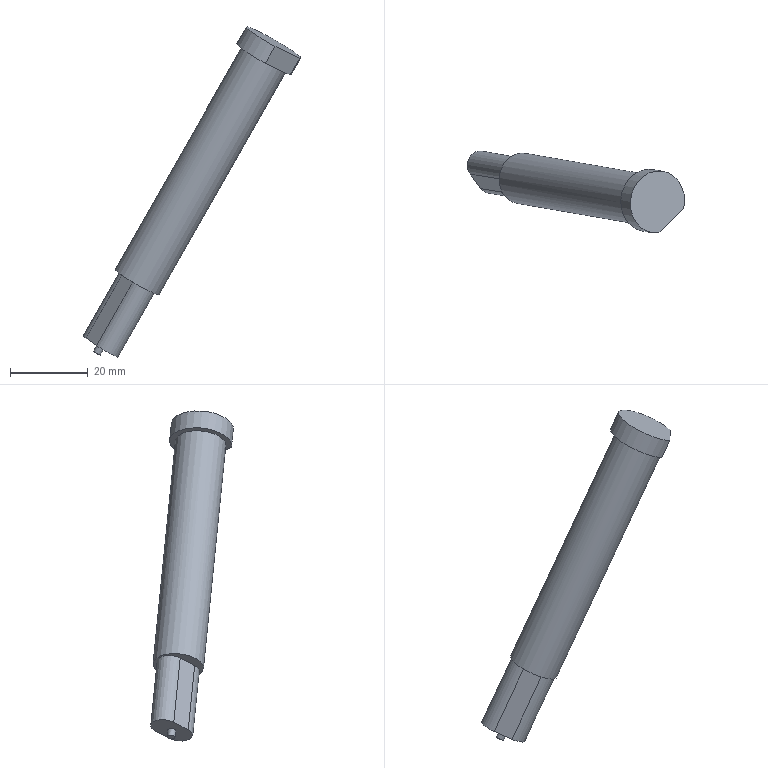Part | NX | features solid 2 | 1 solid | 13 faces | box 55.734 x 21.181 x 84.68 mm | volume 11151 mm3 | plane 8 | cylinder 5 | commonest cylinder face diameters 7.1 x2 2 x1 13 x1 16 x1
STEP:
#1=CARTESIAN_POINT('',(504.153,-25.25,-36.303));
#2=VERTEX_POINT('',#1);
#3=CARTESIAN_POINT('',(508.56,-20.946,-38.377));
#4=DIRECTION('',(0.4924,-0.08682,0.866));
#5=DIRECTION('',(-0.678,-0.6622,0.3191));
#6=AXIS2_PLACEMENT_3D('',#3,#4,#5);
#7=CIRCLE('',#6,6.5);
#8=EDGE_CURVE('',#2,#2,#7,.T.);
#9=ORIENTED_EDGE('',*,*,#8,.F.);
#10=EDGE_LOOP('',(#9));
#11=FACE_BOUND('',#10,.T.);
#12=CARTESIAN_POINT('',(507.517,-25.157,-38.206));
#13=VERTEX_POINT('',#12);
#14=CARTESIAN_POINT('',(504.788,-21.436,-36.282));
#15=VERTEX_POINT('',#14);
#16=CARTESIAN_POINT('',(506.153,-23.297,-37.244));
#17=DIRECTION('',(-0.5458,0.7442,0.385));
#18=VECTOR('',#17,1000.);
#19=LINE('',#16,#18);
#20=EDGE_CURVE('',#13,#15,#19,.T.);
#21=ORIENTED_EDGE('',*,*,#20,.F.);
#22=CARTESIAN_POINT('',(512.331,-20.455,-40.472));
#23=VERTEX_POINT('',#22);
#24=CARTESIAN_POINT('',(509.924,-22.806,-39.339));
#25=DIRECTION('',(0.4924,-0.08682,0.866));
#26=DIRECTION('',(-0.678,-0.6622,0.3191));
#27=AXIS2_PLACEMENT_3D('',#24,#25,#26);
#28=CIRCLE('',#27,3.55);
#29=EDGE_CURVE('',#13,#23,#28,.T.);
#30=ORIENTED_EDGE('',*,*,#29,.T.);
#31=CARTESIAN_POINT('',(509.602,-16.734,-38.547));
#32=VERTEX_POINT('',#31);
#33=CARTESIAN_POINT('',(510.966,-18.595,-39.51));
#34=DIRECTION('',(-0.5458,0.7442,0.385));
#35=VECTOR('',#34,1000.);
#36=LINE('',#33,#35);
#37=EDGE_CURVE('',#23,#32,#36,.T.);
#38=ORIENTED_EDGE('',*,*,#37,.T.);
#39=CARTESIAN_POINT('',(507.195,-19.085,-37.414));
#40=DIRECTION('',(0.4924,-0.08682,0.866));
#41=DIRECTION('',(-0.678,-0.6622,0.3191));
#42=AXIS2_PLACEMENT_3D('',#39,#40,#41);
#43=CIRCLE('',#42,3.55);
#44=EDGE_CURVE('',#32,#15,#43,.T.);
#45=ORIENTED_EDGE('',*,*,#44,.T.);
#46=EDGE_LOOP('',(#21,#30,#38,#45));
#47=FACE_BOUND('',#46,.T.);
#48=CARTESIAN_POINT('',(508.56,-20.946,-38.377));
#49=DIRECTION('',(0.4924,-0.08682,0.866));
#50=DIRECTION('',(-0.678,-0.6622,0.3191));
#51=AXIS2_PLACEMENT_3D('',#48,#49,#50);
#52=PLANE('',#51);
#53=ADVANCED_FACE('',(#11,#47),#52,.F.);
#54=ORIENTED_EDGE('',*,*,#8,.T.);
#55=EDGE_LOOP('',(#54));
#56=FACE_BOUND('',#55,.T.);
#57=CARTESIAN_POINT('',(544.606,-31.514,16.279));
#58=VERTEX_POINT('',#57);
#59=CARTESIAN_POINT('',(541.058,-26.676,18.781));
#60=DIRECTION('',(0.4924,-0.08682,0.866));
#61=DIRECTION('',(-0.5458,0.7442,0.385));
#62=AXIS2_PLACEMENT_3D('',#59,#60,#61);
#63=CIRCLE('',#62,6.5);
#64=EDGE_CURVE('',#58,#58,#63,.T.);
#65=ORIENTED_EDGE('',*,*,#64,.F.);
#66=EDGE_LOOP('',(#65));
#67=FACE_BOUND('',#66,.T.);
#68=CARTESIAN_POINT('',(543.52,-27.11,23.111));
#69=DIRECTION('',(-0.4924,0.08682,-0.866));
#70=DIRECTION('',(0.678,0.6622,-0.3191));
#71=AXIS2_PLACEMENT_3D('',#68,#69,#70);
#72=CYLINDRICAL_SURFACE('',#71,6.5);
#73=ADVANCED_FACE('',(#56,#67),#72,.T.);
#74=CARTESIAN_POINT('',(547.768,-28.425,14.791));
#75=VERTEX_POINT('',#74);
#76=CARTESIAN_POINT('',(541.444,-34.602,17.767));
#77=VERTEX_POINT('',#76);
#78=CARTESIAN_POINT('',(541.058,-26.676,18.781));
#79=DIRECTION('',(0.4924,-0.08682,0.866));
#80=DIRECTION('',(-0.5458,0.7442,0.385));
#81=AXIS2_PLACEMENT_3D('',#78,#79,#80);
#82=CIRCLE('',#81,8.);
#83=EDGE_CURVE('',#75,#77,#82,.T.);
#84=ORIENTED_EDGE('',*,*,#83,.F.);
#85=CARTESIAN_POINT('',(544.606,-31.514,16.279));
#86=DIRECTION('',(-0.678,-0.6622,0.3191));
#87=VECTOR('',#86,1000.);
#88=LINE('',#85,#87);
#89=EDGE_CURVE('',#75,#58,#88,.T.);
#90=ORIENTED_EDGE('',*,*,#89,.T.);
#91=ORIENTED_EDGE('',*,*,#64,.T.);
#92=CARTESIAN_POINT('',(544.606,-31.514,16.279));
#93=DIRECTION('',(-0.678,-0.6622,0.3191));
#94=VECTOR('',#93,1000.);
#95=LINE('',#92,#94);
#96=EDGE_CURVE('',#58,#77,#95,.T.);
#97=ORIENTED_EDGE('',*,*,#96,.T.);
#98=EDGE_LOOP('',(#84,#90,#91,#97));
#99=FACE_BOUND('',#98,.T.);
#100=CARTESIAN_POINT('',(541.058,-26.676,18.781));
#101=DIRECTION('',(0.4924,-0.08682,0.866));
#102=DIRECTION('',(-0.5458,0.7442,0.385));
#103=AXIS2_PLACEMENT_3D('',#100,#101,#102);
#104=PLANE('',#103);
#105=ADVANCED_FACE('',(#99),#104,.F.);
#106=CARTESIAN_POINT('',(543.906,-35.036,22.097));
#107=VERTEX_POINT('',#106);
#108=CARTESIAN_POINT('',(545.876,-35.383,25.561));
#109=DIRECTION('',(-0.4924,0.08682,-0.866));
#110=VECTOR('',#109,1000.);
#111=LINE('',#108,#110);
#112=EDGE_CURVE('',#107,#77,#111,.T.);
#113=ORIENTED_EDGE('',*,*,#112,.F.);
#114=CARTESIAN_POINT('',(550.23,-28.859,19.121));
#115=VERTEX_POINT('',#114);
#116=CARTESIAN_POINT('',(543.52,-27.11,23.111));
#117=DIRECTION('',(0.4924,-0.08682,0.866));
#118=DIRECTION('',(-0.5458,0.7442,0.385));
#119=AXIS2_PLACEMENT_3D('',#116,#117,#118);
#120=CIRCLE('',#119,8.);
#121=EDGE_CURVE('',#115,#107,#120,.T.);
#122=ORIENTED_EDGE('',*,*,#121,.F.);
#123=CARTESIAN_POINT('',(552.199,-29.206,22.585));
#124=DIRECTION('',(-0.4924,0.08682,-0.866));
#125=VECTOR('',#124,1000.);
#126=LINE('',#123,#125);
#127=EDGE_CURVE('',#75,#115,#126,.F.);
#128=ORIENTED_EDGE('',*,*,#127,.F.);
#129=ORIENTED_EDGE('',*,*,#83,.T.);
#130=EDGE_LOOP('',(#113,#122,#128,#129));
#131=FACE_BOUND('',#130,.T.);
#132=CARTESIAN_POINT('',(541.058,-26.676,18.781));
#133=DIRECTION('',(0.4924,-0.08682,0.866));
#134=DIRECTION('',(-0.5458,0.7442,0.385));
#135=AXIS2_PLACEMENT_3D('',#132,#133,#134);
#136=CYLINDRICAL_SURFACE('',#135,8.);
#137=ADVANCED_FACE('',(#131),#136,.T.);
#138=CARTESIAN_POINT('',(547.068,-31.948,20.609));
#139=DIRECTION('',(-0.678,-0.6622,0.3191));
#140=VECTOR('',#139,1000.);
#141=LINE('',#138,#140);
#142=EDGE_CURVE('',#115,#107,#141,.T.);
#143=ORIENTED_EDGE('',*,*,#142,.F.);
#144=ORIENTED_EDGE('',*,*,#121,.T.);
#145=EDGE_LOOP('',(#143,#144));
#146=FACE_BOUND('',#145,.T.);
#147=CARTESIAN_POINT('',(543.52,-27.11,23.111));
#148=DIRECTION('',(0.4924,-0.08682,0.866));
#149=DIRECTION('',(-0.5458,0.7442,0.385));
#150=AXIS2_PLACEMENT_3D('',#147,#148,#149);
#151=PLANE('',#150);
#152=ADVANCED_FACE('',(#146),#151,.T.);
#153=ORIENTED_EDGE('',*,*,#127,.T.);
#154=ORIENTED_EDGE('',*,*,#142,.T.);
#155=ORIENTED_EDGE('',*,*,#112,.T.);
#156=ORIENTED_EDGE('',*,*,#96,.F.);
#157=ORIENTED_EDGE('',*,*,#89,.F.);
#158=EDGE_LOOP('',(#153,#154,#155,#156,#157));
#159=FACE_BOUND('',#158,.T.);
#160=CARTESIAN_POINT('',(545.876,-35.383,25.561));
#161=DIRECTION('',(-0.5458,0.7442,0.385));
#162=DIRECTION('',(-0.4924,0.08682,-0.866));
#163=AXIS2_PLACEMENT_3D('',#160,#161,#162);
#164=PLANE('',#163);
#165=ADVANCED_FACE('',(#159),#164,.F.);
#166=CARTESIAN_POINT('',(498.162,-23.508,-54.661));
#167=VERTEX_POINT('',#166);
#168=CARTESIAN_POINT('',(498.162,-23.508,-54.661));
#169=DIRECTION('',(0.4924,-0.08682,0.866));
#170=VECTOR('',#169,1000.);
#171=LINE('',#168,#170);
#172=EDGE_CURVE('',#167,#13,#171,.T.);
#173=ORIENTED_EDGE('',*,*,#172,.T.);
#174=ORIENTED_EDGE('',*,*,#20,.T.);
#175=CARTESIAN_POINT('',(495.433,-19.786,-52.736));
#176=VERTEX_POINT('',#175);
#177=CARTESIAN_POINT('',(495.433,-19.786,-52.736));
#178=DIRECTION('',(0.4924,-0.08682,0.866));
#179=VECTOR('',#178,1000.);
#180=LINE('',#177,#179);
#181=EDGE_CURVE('',#176,#15,#180,.T.);
#182=ORIENTED_EDGE('',*,*,#181,.F.);
#183=CARTESIAN_POINT('',(498.162,-23.508,-54.661));
#184=DIRECTION('',(-0.5458,0.7442,0.385));
#185=VECTOR('',#184,1000.);
#186=LINE('',#183,#185);
#187=EDGE_CURVE('',#167,#176,#186,.T.);
#188=ORIENTED_EDGE('',*,*,#187,.F.);
#189=EDGE_LOOP('',(#173,#174,#182,#188));
#190=FACE_BOUND('',#189,.T.);
#191=CARTESIAN_POINT('',(498.162,-23.508,-54.661));
#192=DIRECTION('',(0.678,0.6622,-0.3191));
#193=DIRECTION('',(0.4924,-0.08682,0.866));
#194=AXIS2_PLACEMENT_3D('',#191,#192,#193);
#195=PLANE('',#194);
#196=ADVANCED_FACE('',(#190),#195,.F.);
#197=ORIENTED_EDGE('',*,*,#44,.F.);
#198=CARTESIAN_POINT('',(500.246,-15.084,-55.002));
#199=VERTEX_POINT('',#198);
#200=CARTESIAN_POINT('',(500.246,-15.084,-55.002));
#201=DIRECTION('',(0.4924,-0.08682,0.866));
#202=VECTOR('',#201,1000.);
#203=LINE('',#200,#202);
#204=EDGE_CURVE('',#199,#32,#203,.T.);
#205=ORIENTED_EDGE('',*,*,#204,.F.);
#206=CARTESIAN_POINT('',(497.839,-17.435,-53.869));
#207=DIRECTION('',(0.4924,-0.08682,0.866));
#208=DIRECTION('',(-0.678,-0.6622,0.3191));
#209=AXIS2_PLACEMENT_3D('',#206,#207,#208);
#210=CIRCLE('',#209,3.55);
#211=EDGE_CURVE('',#199,#176,#210,.T.);
#212=ORIENTED_EDGE('',*,*,#211,.T.);
#213=ORIENTED_EDGE('',*,*,#181,.T.);
#214=EDGE_LOOP('',(#197,#205,#212,#213));
#215=FACE_BOUND('',#214,.T.);
#216=CARTESIAN_POINT('',(497.839,-17.435,-53.869));
#217=DIRECTION('',(0.4924,-0.08682,0.866));
#218=DIRECTION('',(-0.678,-0.6622,0.3191));
#219=AXIS2_PLACEMENT_3D('',#216,#217,#218);
#220=CYLINDRICAL_SURFACE('',#219,3.55);
#221=ADVANCED_FACE('',(#215),#220,.T.);
#222=ORIENTED_EDGE('',*,*,#37,.F.);
#223=CARTESIAN_POINT('',(502.975,-18.806,-56.926));
#224=VERTEX_POINT('',#223);
#225=CARTESIAN_POINT('',(502.975,-18.806,-56.926));
#226=DIRECTION('',(0.4924,-0.08682,0.866));
#227=VECTOR('',#226,1000.);
#228=LINE('',#225,#227);
#229=EDGE_CURVE('',#224,#23,#228,.T.);
#230=ORIENTED_EDGE('',*,*,#229,.F.);
#231=CARTESIAN_POINT('',(502.975,-18.806,-56.926));
#232=DIRECTION('',(-0.5458,0.7442,0.385));
#233=VECTOR('',#232,1000.);
#234=LINE('',#231,#233);
#235=EDGE_CURVE('',#224,#199,#234,.T.);
#236=ORIENTED_EDGE('',*,*,#235,.T.);
#237=ORIENTED_EDGE('',*,*,#204,.T.);
#238=EDGE_LOOP('',(#222,#230,#236,#237));
#239=FACE_BOUND('',#238,.T.);
#240=CARTESIAN_POINT('',(502.975,-18.806,-56.926));
#241=DIRECTION('',(0.678,0.6622,-0.3191));
#242=DIRECTION('',(0.4924,-0.08682,0.866));
#243=AXIS2_PLACEMENT_3D('',#240,#241,#242);
#244=PLANE('',#243);
#245=ADVANCED_FACE('',(#239),#244,.T.);
#246=ORIENTED_EDGE('',*,*,#29,.F.);
#247=ORIENTED_EDGE('',*,*,#172,.F.);
#248=CARTESIAN_POINT('',(500.568,-21.157,-55.794));
#249=DIRECTION('',(0.4924,-0.08682,0.866));
#250=DIRECTION('',(-0.678,-0.6622,0.3191));
#251=AXIS2_PLACEMENT_3D('',#248,#249,#250);
#252=CIRCLE('',#251,3.55);
#253=EDGE_CURVE('',#167,#224,#252,.T.);
#254=ORIENTED_EDGE('',*,*,#253,.T.);
#255=ORIENTED_EDGE('',*,*,#229,.T.);
#256=EDGE_LOOP('',(#246,#247,#254,#255));
#257=FACE_BOUND('',#256,.T.);
#258=CARTESIAN_POINT('',(500.568,-21.157,-55.794));
#259=DIRECTION('',(0.4924,-0.08682,0.866));
#260=DIRECTION('',(-0.678,-0.6622,0.3191));
#261=AXIS2_PLACEMENT_3D('',#258,#259,#260);
#262=CYLINDRICAL_SURFACE('',#261,3.55);
#263=ADVANCED_FACE('',(#257),#262,.T.);
#264=CARTESIAN_POINT('',(498.526,-19.958,-54.512));
#265=VERTEX_POINT('',#264);
#266=CARTESIAN_POINT('',(499.204,-19.296,-54.831));
#267=DIRECTION('',(0.4924,-0.08682,0.866));
#268=DIRECTION('',(-0.678,-0.6622,0.3191));
#269=AXIS2_PLACEMENT_3D('',#266,#267,#268);
#270=CIRCLE('',#269,1.);
#271=EDGE_CURVE('',#265,#265,#270,.T.);
#272=ORIENTED_EDGE('',*,*,#271,.T.);
#273=EDGE_LOOP('',(#272));
#274=FACE_BOUND('',#273,.T.);
#275=ORIENTED_EDGE('',*,*,#187,.T.);
#276=ORIENTED_EDGE('',*,*,#211,.F.);
#277=ORIENTED_EDGE('',*,*,#235,.F.);
#278=ORIENTED_EDGE('',*,*,#253,.F.);
#279=EDGE_LOOP('',(#275,#276,#277,#278));
#280=FACE_BOUND('',#279,.T.);
#281=CARTESIAN_POINT('',(497.839,-17.435,-53.869));
#282=DIRECTION('',(0.4924,-0.08682,0.866));
#283=DIRECTION('',(-0.678,-0.6622,0.3191));
#284=AXIS2_PLACEMENT_3D('',#281,#282,#283);
#285=PLANE('',#284);
#286=ADVANCED_FACE('',(#274,#280),#285,.F.);
#287=CARTESIAN_POINT('',(497.541,-19.785,-56.244));
#288=VERTEX_POINT('',#287);
#289=CARTESIAN_POINT('',(498.219,-19.122,-56.563));
#290=DIRECTION('',(0.4924,-0.08682,0.866));
#291=DIRECTION('',(-0.678,-0.6622,0.3191));
#292=AXIS2_PLACEMENT_3D('',#289,#290,#291);
#293=CIRCLE('',#292,1.);
#294=EDGE_CURVE('',#288,#288,#293,.T.);
#295=ORIENTED_EDGE('',*,*,#294,.T.);
#296=EDGE_LOOP('',(#295));
#297=FACE_BOUND('',#296,.T.);
#298=ORIENTED_EDGE('',*,*,#271,.F.);
#299=EDGE_LOOP('',(#298));
#300=FACE_BOUND('',#299,.T.);
#301=CARTESIAN_POINT('',(498.219,-19.122,-56.563));
#302=DIRECTION('',(0.4924,-0.08682,0.866));
#303=DIRECTION('',(-0.678,-0.6622,0.3191));
#304=AXIS2_PLACEMENT_3D('',#301,#302,#303);
#305=CYLINDRICAL_SURFACE('',#304,1.);
#306=ADVANCED_FACE('',(#297,#300),#305,.T.);
#307=ORIENTED_EDGE('',*,*,#294,.F.);
#308=EDGE_LOOP('',(#307));
#309=FACE_BOUND('',#308,.T.);
#310=CARTESIAN_POINT('',(498.219,-19.122,-56.563));
#311=DIRECTION('',(0.4924,-0.08682,0.866));
#312=DIRECTION('',(-0.678,-0.6622,0.3191));
#313=AXIS2_PLACEMENT_3D('',#310,#311,#312);
#314=PLANE('',#313);
#315=ADVANCED_FACE('',(#309),#314,.F.);
#316=CLOSED_SHELL('',(#53,#73,#105,#137,#152,#165,#196,#221,#245,#263,#286,#306,#315));
#317=MANIFOLD_SOLID_BREP('',#316);
#318=(LENGTH_UNIT()NAMED_UNIT(*)SI_UNIT(.MILLI.,.METRE.));
#319=UNCERTAINTY_MEASURE_WITH_UNIT(LENGTH_MEASURE(0.00001),#318,'','');
#320=(NAMED_UNIT(*)PLANE_ANGLE_UNIT()SI_UNIT($,.RADIAN.));
#321=(NAMED_UNIT(*)SI_UNIT($,.STERADIAN.)SOLID_ANGLE_UNIT());
#322=(GEOMETRIC_REPRESENTATION_CONTEXT(3)GLOBAL_UNCERTAINTY_ASSIGNED_CONTEXT((#319))GLOBAL_UNIT_ASSIGNED_CONTEXT((#318,#320,#321))REPRESENTATION_CONTEXT('',''));
#323=ADVANCED_BREP_SHAPE_REPRESENTATION('',(#317),#322);